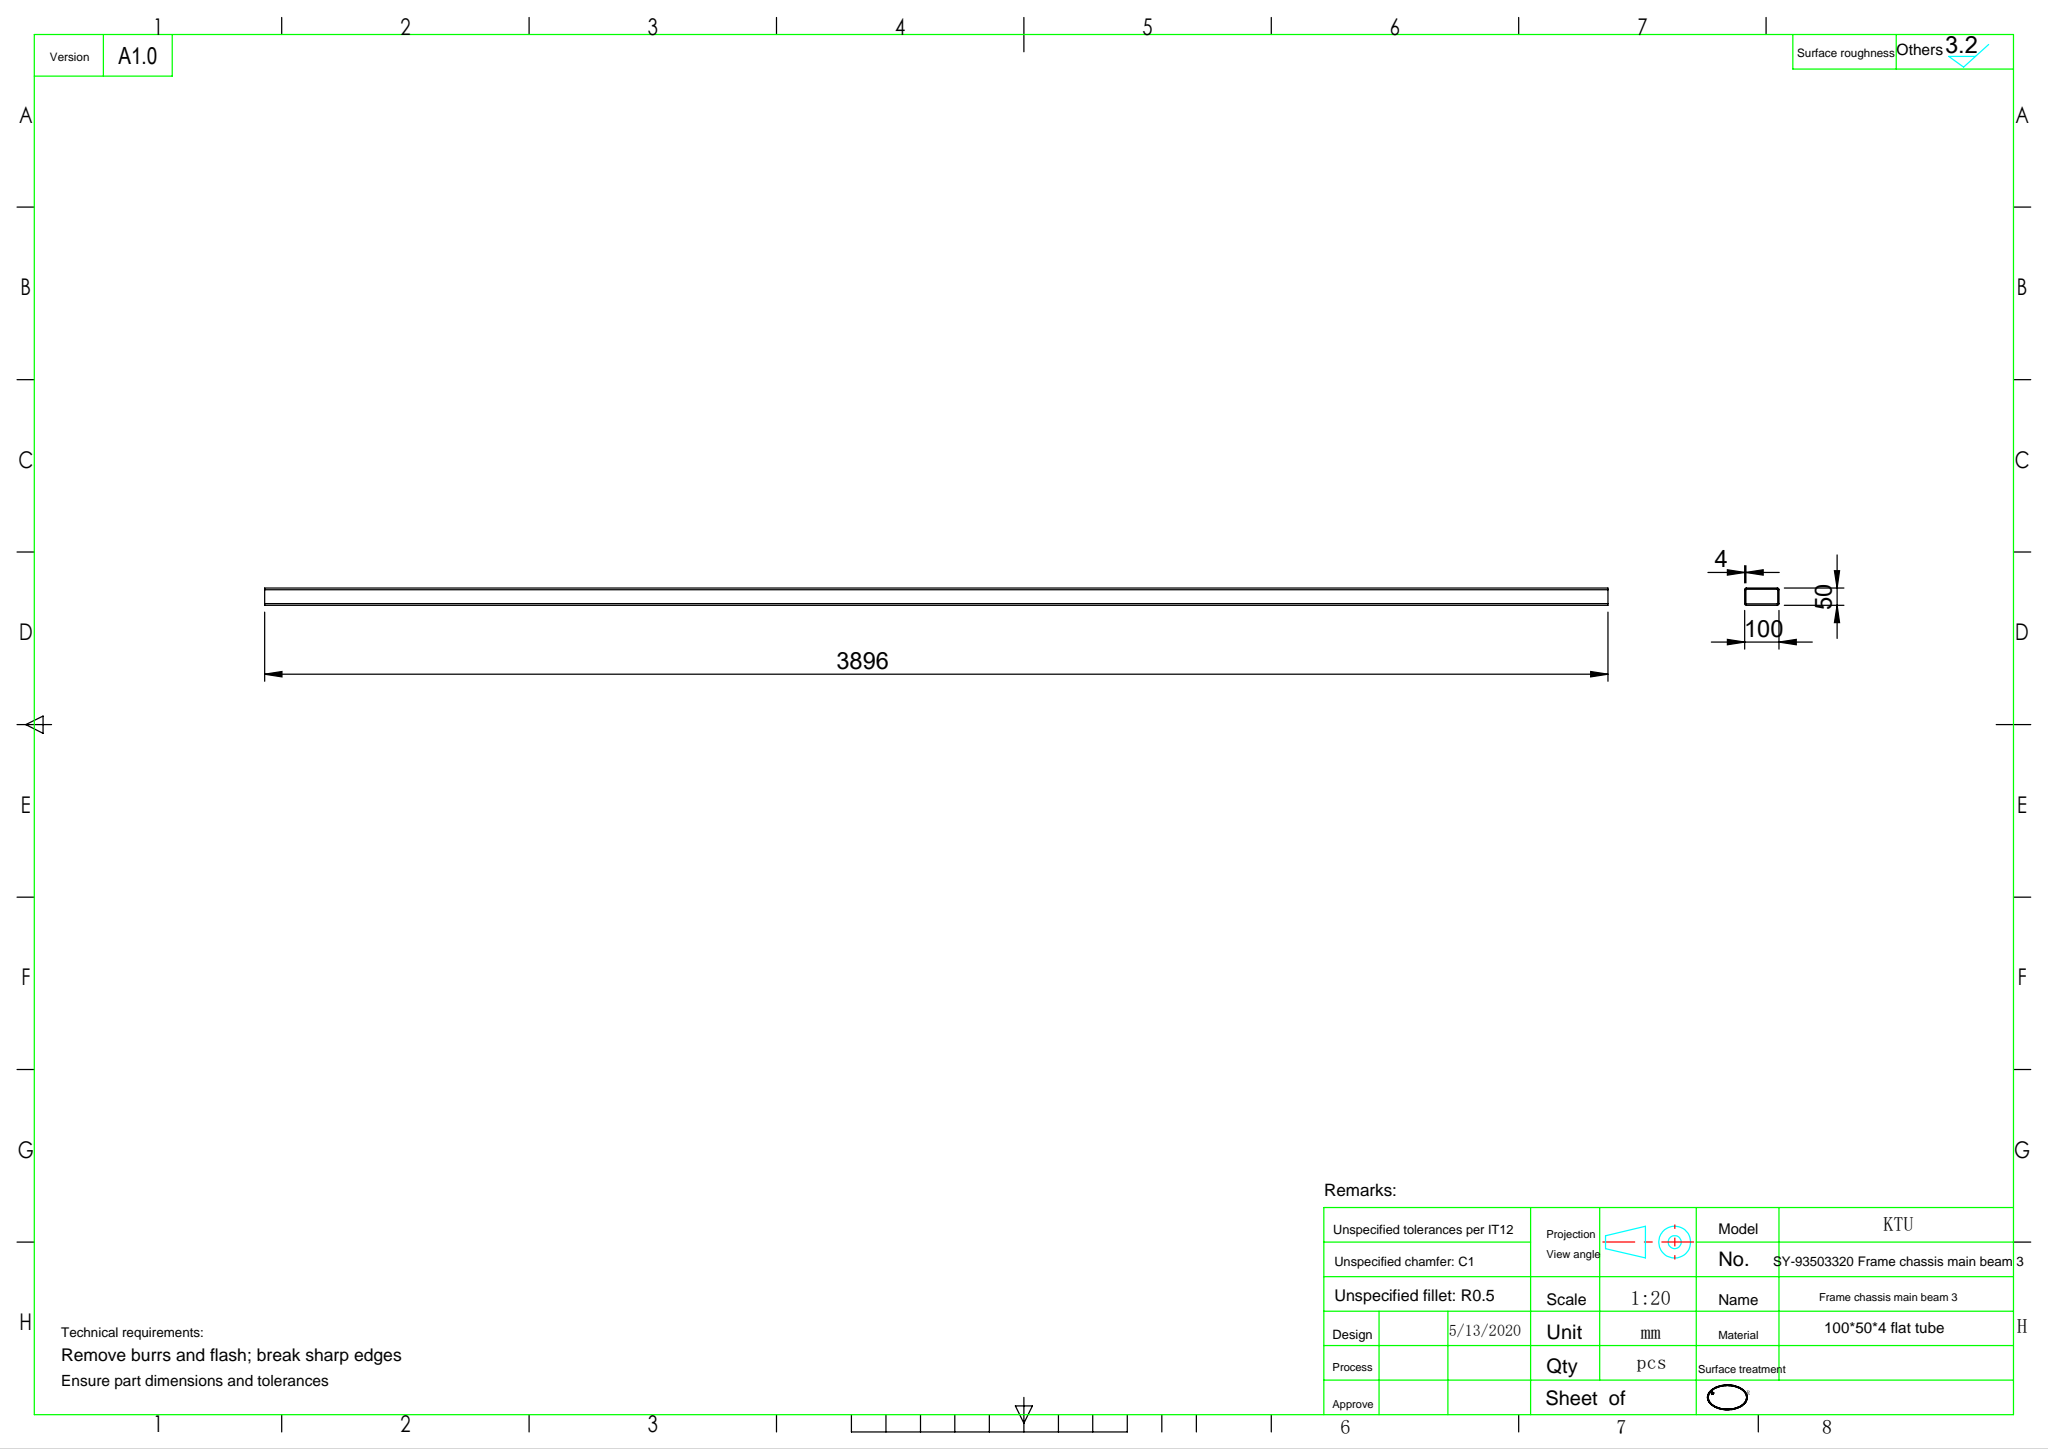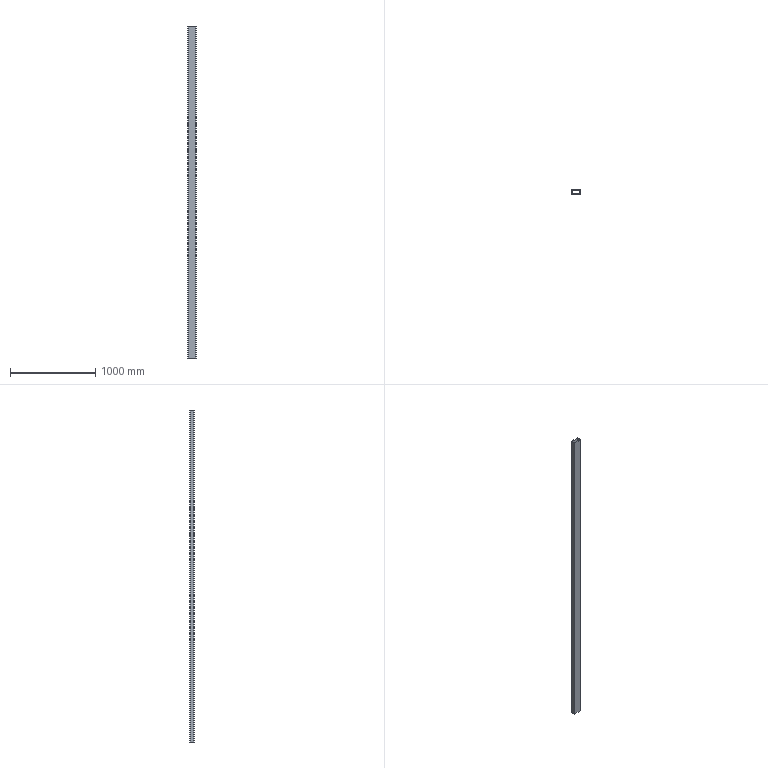Part | SolidWorks | features ExtruThin 1 | 1 solid | 18 faces | box 100 x 50 x 3896 mm | volume 4345591 mm3 | plane 10 | cylinder 8 | commonest cylinder face diameters 2 x4 10 x4
STEP:
#1=CARTESIAN_POINT('',(45.,-25.,1948.));
#2=VERTEX_POINT('',#1);
#3=CARTESIAN_POINT('',(50.,-20.,1948.));
#4=VERTEX_POINT('',#3);
#5=CARTESIAN_POINT('',(45.,-20.,1948.));
#6=DIRECTION('',(0.,0.,1.));
#7=DIRECTION('',(1.,0.,0.));
#8=AXIS2_PLACEMENT_3D('',#5,#6,#7);
#9=CIRCLE('',#8,5.);
#10=EDGE_CURVE('',#2,#4,#9,.T.);
#11=ORIENTED_EDGE('',*,*,#10,.T.);
#12=CARTESIAN_POINT('',(50.,20.,1948.));
#13=VERTEX_POINT('',#12);
#14=CARTESIAN_POINT('',(50.,20.,1948.));
#15=DIRECTION('',(0.,1.,0.));
#16=VECTOR('',#15,1000.);
#17=LINE('',#14,#16);
#18=EDGE_CURVE('',#4,#13,#17,.T.);
#19=ORIENTED_EDGE('',*,*,#18,.T.);
#20=CARTESIAN_POINT('',(45.,25.,1948.));
#21=VERTEX_POINT('',#20);
#22=CARTESIAN_POINT('',(45.,20.,1948.));
#23=DIRECTION('',(0.,0.,1.));
#24=DIRECTION('',(-1.,0.,0.));
#25=AXIS2_PLACEMENT_3D('',#22,#23,#24);
#26=CIRCLE('',#25,5.);
#27=EDGE_CURVE('',#13,#21,#26,.T.);
#28=ORIENTED_EDGE('',*,*,#27,.T.);
#29=CARTESIAN_POINT('',(-45.,25.,1948.));
#30=VERTEX_POINT('',#29);
#31=CARTESIAN_POINT('',(-45.,25.,1948.));
#32=DIRECTION('',(-1.,0.,0.));
#33=VECTOR('',#32,1000.);
#34=LINE('',#31,#33);
#35=EDGE_CURVE('',#21,#30,#34,.T.);
#36=ORIENTED_EDGE('',*,*,#35,.T.);
#37=CARTESIAN_POINT('',(-50.,20.,1948.));
#38=VERTEX_POINT('',#37);
#39=CARTESIAN_POINT('',(-45.,20.,1948.));
#40=DIRECTION('',(0.,0.,1.));
#41=DIRECTION('',(1.,0.,0.));
#42=AXIS2_PLACEMENT_3D('',#39,#40,#41);
#43=CIRCLE('',#42,5.);
#44=EDGE_CURVE('',#30,#38,#43,.T.);
#45=ORIENTED_EDGE('',*,*,#44,.T.);
#46=CARTESIAN_POINT('',(-50.,-20.,1948.));
#47=VERTEX_POINT('',#46);
#48=CARTESIAN_POINT('',(-50.,20.,1948.));
#49=DIRECTION('',(0.,-1.,0.));
#50=VECTOR('',#49,1000.);
#51=LINE('',#48,#50);
#52=EDGE_CURVE('',#38,#47,#51,.T.);
#53=ORIENTED_EDGE('',*,*,#52,.T.);
#54=CARTESIAN_POINT('',(-45.,-25.,1948.));
#55=VERTEX_POINT('',#54);
#56=CARTESIAN_POINT('',(-45.,-20.,1948.));
#57=DIRECTION('',(0.,0.,1.));
#58=DIRECTION('',(1.,0.,0.));
#59=AXIS2_PLACEMENT_3D('',#56,#57,#58);
#60=CIRCLE('',#59,5.);
#61=EDGE_CURVE('',#47,#55,#60,.T.);
#62=ORIENTED_EDGE('',*,*,#61,.T.);
#63=CARTESIAN_POINT('',(-45.,-25.,1948.));
#64=DIRECTION('',(1.,0.,0.));
#65=VECTOR('',#64,1000.);
#66=LINE('',#63,#65);
#67=EDGE_CURVE('',#55,#2,#66,.T.);
#68=ORIENTED_EDGE('',*,*,#67,.T.);
#69=EDGE_LOOP('',(#11,#19,#28,#36,#45,#53,#62,#68));
#70=FACE_OUTER_BOUND('',#69,.T.);
#71=CARTESIAN_POINT('',(46.,-20.,1948.));
#72=VERTEX_POINT('',#71);
#73=CARTESIAN_POINT('',(46.,20.,1948.));
#74=VERTEX_POINT('',#73);
#75=CARTESIAN_POINT('',(46.,20.,1948.));
#76=DIRECTION('',(0.,1.,0.));
#77=VECTOR('',#76,1000.);
#78=LINE('',#75,#77);
#79=EDGE_CURVE('',#72,#74,#78,.T.);
#80=ORIENTED_EDGE('',*,*,#79,.F.);
#81=CARTESIAN_POINT('',(45.,-21.,1948.));
#82=VERTEX_POINT('',#81);
#83=CARTESIAN_POINT('',(45.,-20.,1948.));
#84=DIRECTION('',(0.,0.,1.));
#85=DIRECTION('',(1.,0.,0.));
#86=AXIS2_PLACEMENT_3D('',#83,#84,#85);
#87=CIRCLE('',#86,1.);
#88=EDGE_CURVE('',#82,#72,#87,.T.);
#89=ORIENTED_EDGE('',*,*,#88,.F.);
#90=CARTESIAN_POINT('',(-45.,-21.,1948.));
#91=VERTEX_POINT('',#90);
#92=CARTESIAN_POINT('',(-45.,-21.,1948.));
#93=DIRECTION('',(1.,0.,0.));
#94=VECTOR('',#93,1000.);
#95=LINE('',#92,#94);
#96=EDGE_CURVE('',#91,#82,#95,.T.);
#97=ORIENTED_EDGE('',*,*,#96,.F.);
#98=CARTESIAN_POINT('',(-46.,-20.,1948.));
#99=VERTEX_POINT('',#98);
#100=CARTESIAN_POINT('',(-45.,-20.,1948.));
#101=DIRECTION('',(0.,0.,1.));
#102=DIRECTION('',(1.,0.,0.));
#103=AXIS2_PLACEMENT_3D('',#100,#101,#102);
#104=CIRCLE('',#103,1.);
#105=EDGE_CURVE('',#99,#91,#104,.T.);
#106=ORIENTED_EDGE('',*,*,#105,.F.);
#107=CARTESIAN_POINT('',(-46.,20.,1948.));
#108=VERTEX_POINT('',#107);
#109=CARTESIAN_POINT('',(-46.,20.,1948.));
#110=DIRECTION('',(0.,-1.,0.));
#111=VECTOR('',#110,1000.);
#112=LINE('',#109,#111);
#113=EDGE_CURVE('',#108,#99,#112,.T.);
#114=ORIENTED_EDGE('',*,*,#113,.F.);
#115=CARTESIAN_POINT('',(-45.,21.,1948.));
#116=VERTEX_POINT('',#115);
#117=CARTESIAN_POINT('',(-45.,20.,1948.));
#118=DIRECTION('',(0.,0.,1.));
#119=DIRECTION('',(1.,0.,0.));
#120=AXIS2_PLACEMENT_3D('',#117,#118,#119);
#121=CIRCLE('',#120,1.);
#122=EDGE_CURVE('',#116,#108,#121,.T.);
#123=ORIENTED_EDGE('',*,*,#122,.F.);
#124=CARTESIAN_POINT('',(45.,21.,1948.));
#125=VERTEX_POINT('',#124);
#126=CARTESIAN_POINT('',(-45.,21.,1948.));
#127=DIRECTION('',(-1.,0.,0.));
#128=VECTOR('',#127,1000.);
#129=LINE('',#126,#128);
#130=EDGE_CURVE('',#125,#116,#129,.T.);
#131=ORIENTED_EDGE('',*,*,#130,.F.);
#132=CARTESIAN_POINT('',(45.,20.,1948.));
#133=DIRECTION('',(0.,0.,1.));
#134=DIRECTION('',(1.,0.,0.));
#135=AXIS2_PLACEMENT_3D('',#132,#133,#134);
#136=CIRCLE('',#135,1.);
#137=EDGE_CURVE('',#74,#125,#136,.T.);
#138=ORIENTED_EDGE('',*,*,#137,.F.);
#139=EDGE_LOOP('',(#80,#89,#97,#106,#114,#123,#131,#138));
#140=FACE_BOUND('',#139,.T.);
#141=CARTESIAN_POINT('',(45.,-20.,1948.));
#142=DIRECTION('',(0.,0.,1.));
#143=DIRECTION('',(1.,0.,0.));
#144=AXIS2_PLACEMENT_3D('',#141,#142,#143);
#145=PLANE('',#144);
#146=ADVANCED_FACE('',(#70,#140),#145,.T.);
#147=CARTESIAN_POINT('',(45.,-25.,-1948.));
#148=VERTEX_POINT('',#147);
#149=CARTESIAN_POINT('',(50.,-20.,-1948.));
#150=VERTEX_POINT('',#149);
#151=CARTESIAN_POINT('',(45.,-20.,-1948.));
#152=DIRECTION('',(0.,0.,1.));
#153=DIRECTION('',(1.,0.,0.));
#154=AXIS2_PLACEMENT_3D('',#151,#152,#153);
#155=CIRCLE('',#154,5.);
#156=EDGE_CURVE('',#148,#150,#155,.T.);
#157=ORIENTED_EDGE('',*,*,#156,.F.);
#158=CARTESIAN_POINT('',(-45.,-25.,-1948.));
#159=VERTEX_POINT('',#158);
#160=CARTESIAN_POINT('',(-45.,-25.,-1948.));
#161=DIRECTION('',(1.,0.,0.));
#162=VECTOR('',#161,1000.);
#163=LINE('',#160,#162);
#164=EDGE_CURVE('',#159,#148,#163,.T.);
#165=ORIENTED_EDGE('',*,*,#164,.F.);
#166=CARTESIAN_POINT('',(-50.,-20.,-1948.));
#167=VERTEX_POINT('',#166);
#168=CARTESIAN_POINT('',(-45.,-20.,-1948.));
#169=DIRECTION('',(0.,0.,1.));
#170=DIRECTION('',(1.,0.,0.));
#171=AXIS2_PLACEMENT_3D('',#168,#169,#170);
#172=CIRCLE('',#171,5.);
#173=EDGE_CURVE('',#167,#159,#172,.T.);
#174=ORIENTED_EDGE('',*,*,#173,.F.);
#175=CARTESIAN_POINT('',(-50.,20.,-1948.));
#176=VERTEX_POINT('',#175);
#177=CARTESIAN_POINT('',(-50.,20.,-1948.));
#178=DIRECTION('',(0.,-1.,0.));
#179=VECTOR('',#178,1000.);
#180=LINE('',#177,#179);
#181=EDGE_CURVE('',#176,#167,#180,.T.);
#182=ORIENTED_EDGE('',*,*,#181,.F.);
#183=CARTESIAN_POINT('',(-45.,25.,-1948.));
#184=VERTEX_POINT('',#183);
#185=CARTESIAN_POINT('',(-45.,20.,-1948.));
#186=DIRECTION('',(0.,0.,1.));
#187=DIRECTION('',(1.,0.,0.));
#188=AXIS2_PLACEMENT_3D('',#185,#186,#187);
#189=CIRCLE('',#188,5.);
#190=EDGE_CURVE('',#184,#176,#189,.T.);
#191=ORIENTED_EDGE('',*,*,#190,.F.);
#192=CARTESIAN_POINT('',(45.,25.,-1948.));
#193=VERTEX_POINT('',#192);
#194=CARTESIAN_POINT('',(-45.,25.,-1948.));
#195=DIRECTION('',(-1.,0.,0.));
#196=VECTOR('',#195,1000.);
#197=LINE('',#194,#196);
#198=EDGE_CURVE('',#193,#184,#197,.T.);
#199=ORIENTED_EDGE('',*,*,#198,.F.);
#200=CARTESIAN_POINT('',(50.,20.,-1948.));
#201=VERTEX_POINT('',#200);
#202=CARTESIAN_POINT('',(45.,20.,-1948.));
#203=DIRECTION('',(0.,0.,1.));
#204=DIRECTION('',(-1.,0.,0.));
#205=AXIS2_PLACEMENT_3D('',#202,#203,#204);
#206=CIRCLE('',#205,5.);
#207=EDGE_CURVE('',#201,#193,#206,.T.);
#208=ORIENTED_EDGE('',*,*,#207,.F.);
#209=CARTESIAN_POINT('',(50.,20.,-1948.));
#210=DIRECTION('',(0.,1.,0.));
#211=VECTOR('',#210,1000.);
#212=LINE('',#209,#211);
#213=EDGE_CURVE('',#150,#201,#212,.T.);
#214=ORIENTED_EDGE('',*,*,#213,.F.);
#215=EDGE_LOOP('',(#157,#165,#174,#182,#191,#199,#208,#214));
#216=FACE_OUTER_BOUND('',#215,.T.);
#217=CARTESIAN_POINT('',(45.,-21.,-1948.));
#218=VERTEX_POINT('',#217);
#219=CARTESIAN_POINT('',(46.,-20.,-1948.));
#220=VERTEX_POINT('',#219);
#221=CARTESIAN_POINT('',(45.,-20.,-1948.));
#222=DIRECTION('',(0.,0.,1.));
#223=DIRECTION('',(1.,0.,0.));
#224=AXIS2_PLACEMENT_3D('',#221,#222,#223);
#225=CIRCLE('',#224,1.);
#226=EDGE_CURVE('',#218,#220,#225,.T.);
#227=ORIENTED_EDGE('',*,*,#226,.T.);
#228=CARTESIAN_POINT('',(46.,20.,-1948.));
#229=VERTEX_POINT('',#228);
#230=CARTESIAN_POINT('',(46.,20.,-1948.));
#231=DIRECTION('',(0.,1.,0.));
#232=VECTOR('',#231,1000.);
#233=LINE('',#230,#232);
#234=EDGE_CURVE('',#220,#229,#233,.T.);
#235=ORIENTED_EDGE('',*,*,#234,.T.);
#236=CARTESIAN_POINT('',(45.,21.,-1948.));
#237=VERTEX_POINT('',#236);
#238=CARTESIAN_POINT('',(45.,20.,-1948.));
#239=DIRECTION('',(0.,0.,1.));
#240=DIRECTION('',(1.,0.,0.));
#241=AXIS2_PLACEMENT_3D('',#238,#239,#240);
#242=CIRCLE('',#241,1.);
#243=EDGE_CURVE('',#229,#237,#242,.T.);
#244=ORIENTED_EDGE('',*,*,#243,.T.);
#245=CARTESIAN_POINT('',(-45.,21.,-1948.));
#246=VERTEX_POINT('',#245);
#247=CARTESIAN_POINT('',(-45.,21.,-1948.));
#248=DIRECTION('',(-1.,0.,0.));
#249=VECTOR('',#248,1000.);
#250=LINE('',#247,#249);
#251=EDGE_CURVE('',#237,#246,#250,.T.);
#252=ORIENTED_EDGE('',*,*,#251,.T.);
#253=CARTESIAN_POINT('',(-46.,20.,-1948.));
#254=VERTEX_POINT('',#253);
#255=CARTESIAN_POINT('',(-45.,20.,-1948.));
#256=DIRECTION('',(0.,0.,1.));
#257=DIRECTION('',(1.,0.,0.));
#258=AXIS2_PLACEMENT_3D('',#255,#256,#257);
#259=CIRCLE('',#258,1.);
#260=EDGE_CURVE('',#246,#254,#259,.T.);
#261=ORIENTED_EDGE('',*,*,#260,.T.);
#262=CARTESIAN_POINT('',(-46.,-20.,-1948.));
#263=VERTEX_POINT('',#262);
#264=CARTESIAN_POINT('',(-46.,20.,-1948.));
#265=DIRECTION('',(0.,-1.,0.));
#266=VECTOR('',#265,1000.);
#267=LINE('',#264,#266);
#268=EDGE_CURVE('',#254,#263,#267,.T.);
#269=ORIENTED_EDGE('',*,*,#268,.T.);
#270=CARTESIAN_POINT('',(-45.,-21.,-1948.));
#271=VERTEX_POINT('',#270);
#272=CARTESIAN_POINT('',(-45.,-20.,-1948.));
#273=DIRECTION('',(0.,0.,1.));
#274=DIRECTION('',(1.,0.,0.));
#275=AXIS2_PLACEMENT_3D('',#272,#273,#274);
#276=CIRCLE('',#275,1.);
#277=EDGE_CURVE('',#263,#271,#276,.T.);
#278=ORIENTED_EDGE('',*,*,#277,.T.);
#279=CARTESIAN_POINT('',(-45.,-21.,-1948.));
#280=DIRECTION('',(1.,0.,0.));
#281=VECTOR('',#280,1000.);
#282=LINE('',#279,#281);
#283=EDGE_CURVE('',#271,#218,#282,.T.);
#284=ORIENTED_EDGE('',*,*,#283,.T.);
#285=EDGE_LOOP('',(#227,#235,#244,#252,#261,#269,#278,#284));
#286=FACE_BOUND('',#285,.T.);
#287=CARTESIAN_POINT('',(45.,-20.,-1948.));
#288=DIRECTION('',(0.,0.,1.));
#289=DIRECTION('',(1.,0.,0.));
#290=AXIS2_PLACEMENT_3D('',#287,#288,#289);
#291=PLANE('',#290);
#292=ADVANCED_FACE('',(#216,#286),#291,.F.);
#293=ORIENTED_EDGE('',*,*,#156,.T.);
#294=CARTESIAN_POINT('',(50.,-20.,1948.));
#295=DIRECTION('',(0.,0.,-1.));
#296=VECTOR('',#295,1000.);
#297=LINE('',#294,#296);
#298=EDGE_CURVE('',#4,#150,#297,.T.);
#299=ORIENTED_EDGE('',*,*,#298,.F.);
#300=ORIENTED_EDGE('',*,*,#10,.F.);
#301=CARTESIAN_POINT('',(45.,-25.,1948.));
#302=DIRECTION('',(0.,0.,-1.));
#303=VECTOR('',#302,1000.);
#304=LINE('',#301,#303);
#305=EDGE_CURVE('',#2,#148,#304,.T.);
#306=ORIENTED_EDGE('',*,*,#305,.T.);
#307=EDGE_LOOP('',(#293,#299,#300,#306));
#308=FACE_OUTER_BOUND('',#307,.T.);
#309=CARTESIAN_POINT('',(45.,-20.,1948.));
#310=DIRECTION('',(0.,0.,-1.));
#311=DIRECTION('',(-1.,0.,0.));
#312=AXIS2_PLACEMENT_3D('',#309,#310,#311);
#313=CYLINDRICAL_SURFACE('',#312,5.);
#314=ADVANCED_FACE('',(#308),#313,.T.);
#315=ORIENTED_EDGE('',*,*,#213,.T.);
#316=CARTESIAN_POINT('',(50.,20.,1948.));
#317=DIRECTION('',(0.,0.,-1.));
#318=VECTOR('',#317,1000.);
#319=LINE('',#316,#318);
#320=EDGE_CURVE('',#13,#201,#319,.T.);
#321=ORIENTED_EDGE('',*,*,#320,.F.);
#322=ORIENTED_EDGE('',*,*,#18,.F.);
#323=ORIENTED_EDGE('',*,*,#298,.T.);
#324=EDGE_LOOP('',(#315,#321,#322,#323));
#325=FACE_OUTER_BOUND('',#324,.T.);
#326=CARTESIAN_POINT('',(50.,20.,1948.));
#327=DIRECTION('',(-1.,0.,0.));
#328=DIRECTION('',(0.,-1.,0.));
#329=AXIS2_PLACEMENT_3D('',#326,#327,#328);
#330=PLANE('',#329);
#331=ADVANCED_FACE('',(#325),#330,.F.);
#332=ORIENTED_EDGE('',*,*,#207,.T.);
#333=CARTESIAN_POINT('',(45.,25.,1948.));
#334=DIRECTION('',(0.,0.,-1.));
#335=VECTOR('',#334,1000.);
#336=LINE('',#333,#335);
#337=EDGE_CURVE('',#21,#193,#336,.T.);
#338=ORIENTED_EDGE('',*,*,#337,.F.);
#339=ORIENTED_EDGE('',*,*,#27,.F.);
#340=ORIENTED_EDGE('',*,*,#320,.T.);
#341=EDGE_LOOP('',(#332,#338,#339,#340));
#342=FACE_OUTER_BOUND('',#341,.T.);
#343=CARTESIAN_POINT('',(45.,20.,1948.));
#344=DIRECTION('',(0.,0.,-1.));
#345=DIRECTION('',(-1.,0.,0.));
#346=AXIS2_PLACEMENT_3D('',#343,#344,#345);
#347=CYLINDRICAL_SURFACE('',#346,5.);
#348=ADVANCED_FACE('',(#342),#347,.T.);
#349=ORIENTED_EDGE('',*,*,#198,.T.);
#350=CARTESIAN_POINT('',(-45.,25.,1948.));
#351=DIRECTION('',(0.,0.,-1.));
#352=VECTOR('',#351,1000.);
#353=LINE('',#350,#352);
#354=EDGE_CURVE('',#30,#184,#353,.T.);
#355=ORIENTED_EDGE('',*,*,#354,.F.);
#356=ORIENTED_EDGE('',*,*,#35,.F.);
#357=ORIENTED_EDGE('',*,*,#337,.T.);
#358=EDGE_LOOP('',(#349,#355,#356,#357));
#359=FACE_OUTER_BOUND('',#358,.T.);
#360=CARTESIAN_POINT('',(-45.,25.,1948.));
#361=DIRECTION('',(0.,-1.,0.));
#362=DIRECTION('',(0.,0.,-1.));
#363=AXIS2_PLACEMENT_3D('',#360,#361,#362);
#364=PLANE('',#363);
#365=ADVANCED_FACE('',(#359),#364,.F.);
#366=ORIENTED_EDGE('',*,*,#190,.T.);
#367=CARTESIAN_POINT('',(-50.,20.,1948.));
#368=DIRECTION('',(0.,0.,-1.));
#369=VECTOR('',#368,1000.);
#370=LINE('',#367,#369);
#371=EDGE_CURVE('',#38,#176,#370,.T.);
#372=ORIENTED_EDGE('',*,*,#371,.F.);
#373=ORIENTED_EDGE('',*,*,#44,.F.);
#374=ORIENTED_EDGE('',*,*,#354,.T.);
#375=EDGE_LOOP('',(#366,#372,#373,#374));
#376=FACE_OUTER_BOUND('',#375,.T.);
#377=CARTESIAN_POINT('',(-45.,20.,1948.));
#378=DIRECTION('',(0.,0.,-1.));
#379=DIRECTION('',(-1.,0.,0.));
#380=AXIS2_PLACEMENT_3D('',#377,#378,#379);
#381=CYLINDRICAL_SURFACE('',#380,5.);
#382=ADVANCED_FACE('',(#376),#381,.T.);
#383=ORIENTED_EDGE('',*,*,#181,.T.);
#384=CARTESIAN_POINT('',(-50.,-20.,1948.));
#385=DIRECTION('',(0.,0.,-1.));
#386=VECTOR('',#385,1000.);
#387=LINE('',#384,#386);
#388=EDGE_CURVE('',#47,#167,#387,.T.);
#389=ORIENTED_EDGE('',*,*,#388,.F.);
#390=ORIENTED_EDGE('',*,*,#52,.F.);
#391=ORIENTED_EDGE('',*,*,#371,.T.);
#392=EDGE_LOOP('',(#383,#389,#390,#391));
#393=FACE_OUTER_BOUND('',#392,.T.);
#394=CARTESIAN_POINT('',(-50.,20.,1948.));
#395=DIRECTION('',(1.,0.,0.));
#396=DIRECTION('',(0.,0.,-1.));
#397=AXIS2_PLACEMENT_3D('',#394,#395,#396);
#398=PLANE('',#397);
#399=ADVANCED_FACE('',(#393),#398,.F.);
#400=ORIENTED_EDGE('',*,*,#173,.T.);
#401=CARTESIAN_POINT('',(-45.,-25.,1948.));
#402=DIRECTION('',(0.,0.,-1.));
#403=VECTOR('',#402,1000.);
#404=LINE('',#401,#403);
#405=EDGE_CURVE('',#55,#159,#404,.T.);
#406=ORIENTED_EDGE('',*,*,#405,.F.);
#407=ORIENTED_EDGE('',*,*,#61,.F.);
#408=ORIENTED_EDGE('',*,*,#388,.T.);
#409=EDGE_LOOP('',(#400,#406,#407,#408));
#410=FACE_OUTER_BOUND('',#409,.T.);
#411=CARTESIAN_POINT('',(-45.,-20.,1948.));
#412=DIRECTION('',(0.,0.,-1.));
#413=DIRECTION('',(-1.,0.,0.));
#414=AXIS2_PLACEMENT_3D('',#411,#412,#413);
#415=CYLINDRICAL_SURFACE('',#414,5.);
#416=ADVANCED_FACE('',(#410),#415,.T.);
#417=ORIENTED_EDGE('',*,*,#164,.T.);
#418=ORIENTED_EDGE('',*,*,#305,.F.);
#419=ORIENTED_EDGE('',*,*,#67,.F.);
#420=ORIENTED_EDGE('',*,*,#405,.T.);
#421=EDGE_LOOP('',(#417,#418,#419,#420));
#422=FACE_OUTER_BOUND('',#421,.T.);
#423=CARTESIAN_POINT('',(-45.,-25.,1948.));
#424=DIRECTION('',(0.,1.,0.));
#425=DIRECTION('',(0.,0.,1.));
#426=AXIS2_PLACEMENT_3D('',#423,#424,#425);
#427=PLANE('',#426);
#428=ADVANCED_FACE('',(#422),#427,.F.);
#429=ORIENTED_EDGE('',*,*,#226,.F.);
#430=CARTESIAN_POINT('',(45.,-21.,1948.));
#431=DIRECTION('',(0.,0.,-1.));
#432=VECTOR('',#431,1000.);
#433=LINE('',#430,#432);
#434=EDGE_CURVE('',#82,#218,#433,.T.);
#435=ORIENTED_EDGE('',*,*,#434,.F.);
#436=ORIENTED_EDGE('',*,*,#88,.T.);
#437=CARTESIAN_POINT('',(46.,-20.,1948.));
#438=DIRECTION('',(0.,0.,-1.));
#439=VECTOR('',#438,1000.);
#440=LINE('',#437,#439);
#441=EDGE_CURVE('',#72,#220,#440,.T.);
#442=ORIENTED_EDGE('',*,*,#441,.T.);
#443=EDGE_LOOP('',(#429,#435,#436,#442));
#444=FACE_OUTER_BOUND('',#443,.T.);
#445=CARTESIAN_POINT('',(45.,-20.,1948.));
#446=DIRECTION('',(0.,0.,-1.));
#447=DIRECTION('',(-1.,0.,0.));
#448=AXIS2_PLACEMENT_3D('',#445,#446,#447);
#449=CYLINDRICAL_SURFACE('',#448,1.);
#450=ADVANCED_FACE('',(#444),#449,.F.);
#451=ORIENTED_EDGE('',*,*,#234,.F.);
#452=ORIENTED_EDGE('',*,*,#441,.F.);
#453=ORIENTED_EDGE('',*,*,#79,.T.);
#454=CARTESIAN_POINT('',(46.,20.,1948.));
#455=DIRECTION('',(0.,0.,-1.));
#456=VECTOR('',#455,1000.);
#457=LINE('',#454,#456);
#458=EDGE_CURVE('',#74,#229,#457,.T.);
#459=ORIENTED_EDGE('',*,*,#458,.T.);
#460=EDGE_LOOP('',(#451,#452,#453,#459));
#461=FACE_OUTER_BOUND('',#460,.T.);
#462=CARTESIAN_POINT('',(46.,20.,1948.));
#463=DIRECTION('',(-1.,0.,0.));
#464=DIRECTION('',(0.,-1.,0.));
#465=AXIS2_PLACEMENT_3D('',#462,#463,#464);
#466=PLANE('',#465);
#467=ADVANCED_FACE('',(#461),#466,.T.);
#468=ORIENTED_EDGE('',*,*,#243,.F.);
#469=ORIENTED_EDGE('',*,*,#458,.F.);
#470=ORIENTED_EDGE('',*,*,#137,.T.);
#471=CARTESIAN_POINT('',(45.,21.,1948.));
#472=DIRECTION('',(0.,0.,-1.));
#473=VECTOR('',#472,1000.);
#474=LINE('',#471,#473);
#475=EDGE_CURVE('',#125,#237,#474,.T.);
#476=ORIENTED_EDGE('',*,*,#475,.T.);
#477=EDGE_LOOP('',(#468,#469,#470,#476));
#478=FACE_OUTER_BOUND('',#477,.T.);
#479=CARTESIAN_POINT('',(45.,20.,1948.));
#480=DIRECTION('',(0.,0.,-1.));
#481=DIRECTION('',(-1.,0.,0.));
#482=AXIS2_PLACEMENT_3D('',#479,#480,#481);
#483=CYLINDRICAL_SURFACE('',#482,1.);
#484=ADVANCED_FACE('',(#478),#483,.F.);
#485=ORIENTED_EDGE('',*,*,#251,.F.);
#486=ORIENTED_EDGE('',*,*,#475,.F.);
#487=ORIENTED_EDGE('',*,*,#130,.T.);
#488=CARTESIAN_POINT('',(-45.,21.,1948.));
#489=DIRECTION('',(0.,0.,-1.));
#490=VECTOR('',#489,1000.);
#491=LINE('',#488,#490);
#492=EDGE_CURVE('',#116,#246,#491,.T.);
#493=ORIENTED_EDGE('',*,*,#492,.T.);
#494=EDGE_LOOP('',(#485,#486,#487,#493));
#495=FACE_OUTER_BOUND('',#494,.T.);
#496=CARTESIAN_POINT('',(-45.,21.,1948.));
#497=DIRECTION('',(0.,-1.,0.));
#498=DIRECTION('',(0.,0.,-1.));
#499=AXIS2_PLACEMENT_3D('',#496,#497,#498);
#500=PLANE('',#499);
#501=ADVANCED_FACE('',(#495),#500,.T.);
#502=ORIENTED_EDGE('',*,*,#260,.F.);
#503=ORIENTED_EDGE('',*,*,#492,.F.);
#504=ORIENTED_EDGE('',*,*,#122,.T.);
#505=CARTESIAN_POINT('',(-46.,20.,1948.));
#506=DIRECTION('',(0.,0.,-1.));
#507=VECTOR('',#506,1000.);
#508=LINE('',#505,#507);
#509=EDGE_CURVE('',#108,#254,#508,.T.);
#510=ORIENTED_EDGE('',*,*,#509,.T.);
#511=EDGE_LOOP('',(#502,#503,#504,#510));
#512=FACE_OUTER_BOUND('',#511,.T.);
#513=CARTESIAN_POINT('',(-45.,20.,1948.));
#514=DIRECTION('',(0.,0.,-1.));
#515=DIRECTION('',(-1.,0.,0.));
#516=AXIS2_PLACEMENT_3D('',#513,#514,#515);
#517=CYLINDRICAL_SURFACE('',#516,1.);
#518=ADVANCED_FACE('',(#512),#517,.F.);
#519=ORIENTED_EDGE('',*,*,#268,.F.);
#520=ORIENTED_EDGE('',*,*,#509,.F.);
#521=ORIENTED_EDGE('',*,*,#113,.T.);
#522=CARTESIAN_POINT('',(-46.,-20.,1948.));
#523=DIRECTION('',(0.,0.,-1.));
#524=VECTOR('',#523,1000.);
#525=LINE('',#522,#524);
#526=EDGE_CURVE('',#99,#263,#525,.T.);
#527=ORIENTED_EDGE('',*,*,#526,.T.);
#528=EDGE_LOOP('',(#519,#520,#521,#527));
#529=FACE_OUTER_BOUND('',#528,.T.);
#530=CARTESIAN_POINT('',(-46.,20.,1948.));
#531=DIRECTION('',(1.,0.,0.));
#532=DIRECTION('',(0.,0.,-1.));
#533=AXIS2_PLACEMENT_3D('',#530,#531,#532);
#534=PLANE('',#533);
#535=ADVANCED_FACE('',(#529),#534,.T.);
#536=ORIENTED_EDGE('',*,*,#277,.F.);
#537=ORIENTED_EDGE('',*,*,#526,.F.);
#538=ORIENTED_EDGE('',*,*,#105,.T.);
#539=CARTESIAN_POINT('',(-45.,-21.,1948.));
#540=DIRECTION('',(0.,0.,-1.));
#541=VECTOR('',#540,1000.);
#542=LINE('',#539,#541);
#543=EDGE_CURVE('',#91,#271,#542,.T.);
#544=ORIENTED_EDGE('',*,*,#543,.T.);
#545=EDGE_LOOP('',(#536,#537,#538,#544));
#546=FACE_OUTER_BOUND('',#545,.T.);
#547=CARTESIAN_POINT('',(-45.,-20.,1948.));
#548=DIRECTION('',(0.,0.,-1.));
#549=DIRECTION('',(-1.,0.,0.));
#550=AXIS2_PLACEMENT_3D('',#547,#548,#549);
#551=CYLINDRICAL_SURFACE('',#550,1.);
#552=ADVANCED_FACE('',(#546),#551,.F.);
#553=ORIENTED_EDGE('',*,*,#283,.F.);
#554=ORIENTED_EDGE('',*,*,#543,.F.);
#555=ORIENTED_EDGE('',*,*,#96,.T.);
#556=ORIENTED_EDGE('',*,*,#434,.T.);
#557=EDGE_LOOP('',(#553,#554,#555,#556));
#558=FACE_OUTER_BOUND('',#557,.T.);
#559=CARTESIAN_POINT('',(-45.,-21.,1948.));
#560=DIRECTION('',(0.,1.,0.));
#561=DIRECTION('',(0.,0.,1.));
#562=AXIS2_PLACEMENT_3D('',#559,#560,#561);
#563=PLANE('',#562);
#564=ADVANCED_FACE('',(#558),#563,.T.);
#565=CLOSED_SHELL('',(#146,#292,#314,#331,#348,#365,#382,#399,#416,#428,#450,#467,#484,#501,#518,#535,#552,#564));
#566=MANIFOLD_SOLID_BREP('',#565);
#567=CARTESIAN_POINT('',(0.,0.,0.));
#568=DIRECTION('',(0.,0.,1.));
#569=DIRECTION('',(1.,0.,0.));
#570=AXIS2_PLACEMENT_3D('',#567,#568,#569);
#571=(LENGTH_UNIT()NAMED_UNIT(*)SI_UNIT(.MILLI.,.METRE.));
#572=UNCERTAINTY_MEASURE_WITH_UNIT(LENGTH_MEASURE(0.00001),#571,'','');
#573=(NAMED_UNIT(*)PLANE_ANGLE_UNIT()SI_UNIT($,.RADIAN.));
#574=(NAMED_UNIT(*)SI_UNIT($,.STERADIAN.)SOLID_ANGLE_UNIT());
#575=(GEOMETRIC_REPRESENTATION_CONTEXT(3)GLOBAL_UNCERTAINTY_ASSIGNED_CONTEXT((#572))GLOBAL_UNIT_ASSIGNED_CONTEXT((#571,#573,#574))REPRESENTATION_CONTEXT('',''));
#576=ADVANCED_BREP_SHAPE_REPRESENTATION('',(#566,#570),#575);